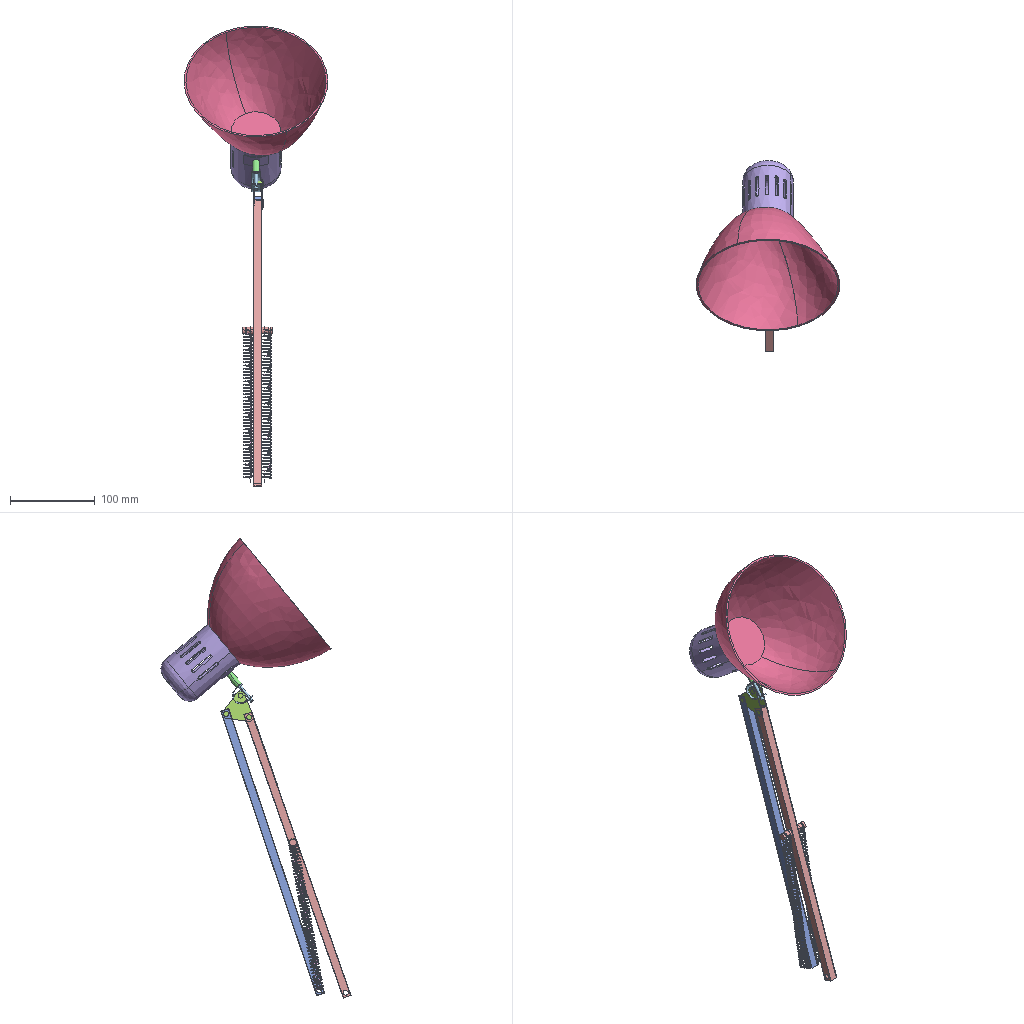Assembly | SolidWorks | 8 different items | 9 placed | box 170 x 225 x 544 mm
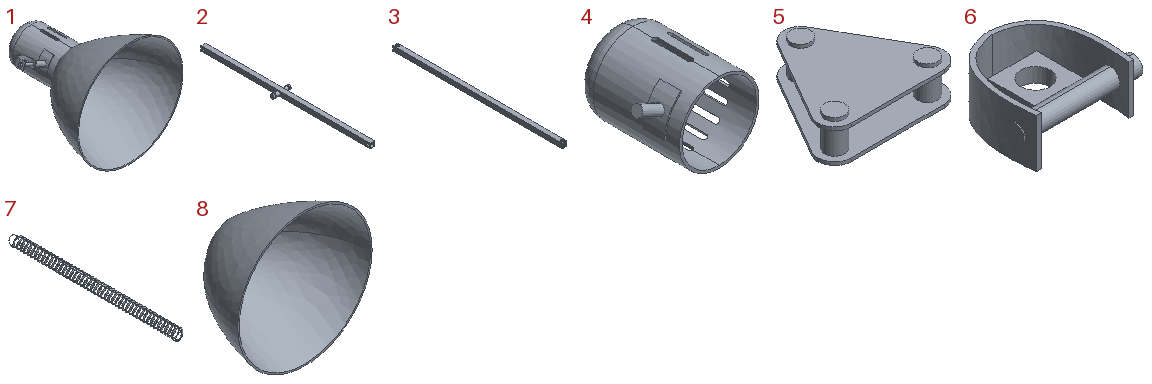Parts list (item | name | quantity | parent item | size | volume | features):
1 | (subassembly) | x1 | - | 170 x 174.745 x 170 mm | 120724 mm3 | features CompositeCurve 4
2 | - | x1 | - | 36 x 355 x 10 mm | 7907 mm3 | features ICE 5, Extrusion 1, MirrorSolid 1
3 | - | x1 | - | 10 x 355 x 10 mm | 6688 mm3 | features ICE 2, Extrusion 1
4 | - | x1 | in 1 | 76.1 x 80 x 60 mm | 29738 mm3 | features ICE 4, CirPattern 1, Extrusion 1, Fillet 1, Shell 1
5 | - | x1 | - | 37.679 x 33.971 x 12 mm | 2499 mm3 | features ICE 2, Extrusion 1, MirrorPattern 1
6 | - | x1 | in 1 | 24.5 x 20 x 10 mm | 968.354 mm3 | features ICE 4, Extrusion 1
7 | - | x2 | - | 10.978 x 187.418 x 11.39 mm | 1153 mm3 | features Helix 1, ICE 1, MirrorSolid 1, Sweep 1
8 | - | x1 | in 1 | 170 x 94.745 x 170 mm | 90040 mm3 | features Blend 1, Shell 1
Mates (type | each side: item.copy, entity, surface, feature):
In the top assembly
Concentric | assembly face | assembly face | 4 times
Parallel | assembly face | assembly face | 3 times
Coincident | assembly face | assembly face | 3 times
Concentric | assembly face | 2.1 face cylinder Cut-Extrude1
Coincident | assembly face | 2.1 face plane Boss-Extrude1
Concentric | assembly face | 3.1 face cylinder Cut-Extrude1
Coincident | assembly face | 3.1 face plane Boss-Extrude1
Concentric | 3.1 face cylinder Cut-Extrude2 | 5.1 face cylinder Boss-Extrude2
Coincident | 3.1 face plane Boss-Extrude1 | 5.1 face plane Boss-Extrude1
Concentric | 2.1 face cylinder Cut-Extrude2 | 5.1 face cylinder Boss-Extrude2
Concentric | assembly face | assembly edge
Concentric | assembly face | 7.1 edge | 2 times
Concentric | 2.1 face cylinder Boss-Extrude3 | 7.1 edge
Concentric | 2.1 face cylinder Boss-Extrude2 | 7.1 edge
Concentric | 5.1 face cylinder Boss-Extrude2 | 6.1 face cylinder Cut-Extrude1
Coincident | 5.1 face plane Mirror3 | 6.1 face plane Boss-Extrude4
In subassembly 1
Coincident | 4.1 edge | 8.1 edge
Coincident | 4.1 face plane Boss-Extrude5 | 6.2 face plane Boss-Extrude3
Concentric | 4.1 edge | 6.2 edge
Parallel | 8.1 face plane Loft1 | 6.2 face plane Boss-Extrude1